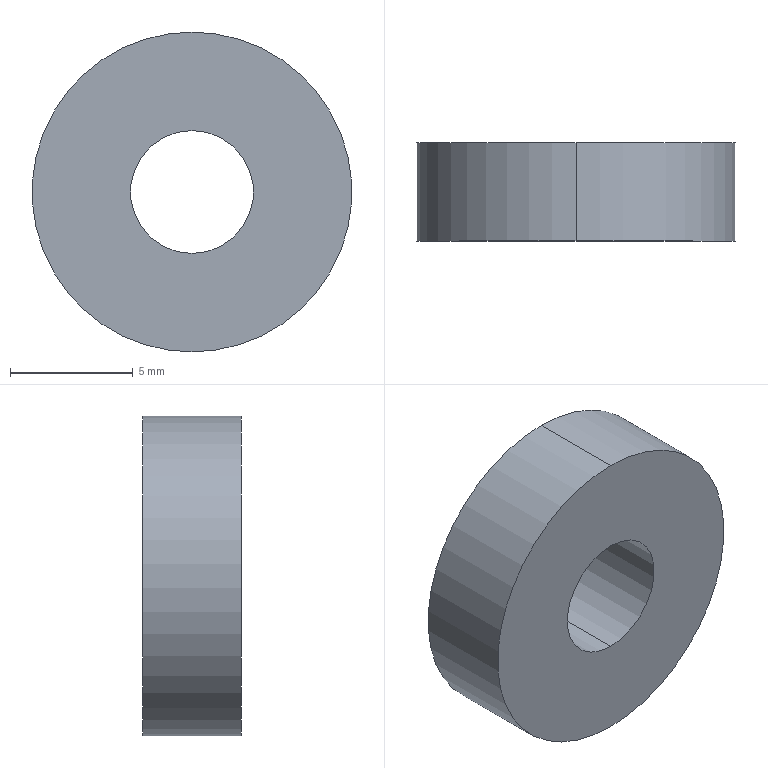Part | NX | 1 solid | 6 faces | box 13 x 4 x 13 mm | volume 452.389 mm3 | cylinder 4 | plane 2 | commonest cylinder face diameters 5 x2 13 x2
STEP:
#1=CARTESIAN_POINT('',(-123.5,286.7,-39.863));
#2=VERTEX_POINT('',#1);
#3=CARTESIAN_POINT('',(-123.5,286.7,-44.863));
#4=VERTEX_POINT('',#3);
#5=CARTESIAN_POINT('',(-123.5,286.7,-42.363));
#6=DIRECTION('',(0.,1.,0.));
#7=DIRECTION('',(0.,0.,1.));
#8=AXIS2_PLACEMENT_3D('',#5,#6,#7);
#9=CIRCLE('',#8,2.5);
#10=EDGE_CURVE('',#2,#4,#9,.T.);
#11=ORIENTED_EDGE('',*,*,#10,.F.);
#12=CARTESIAN_POINT('',(-123.5,290.7,-39.863));
#13=VERTEX_POINT('',#12);
#14=CARTESIAN_POINT('',(-123.5,290.7,-39.863));
#15=DIRECTION('',(0.,1.,0.));
#16=VECTOR('',#15,1000.);
#17=LINE('',#14,#16);
#18=EDGE_CURVE('',#2,#13,#17,.T.);
#19=ORIENTED_EDGE('',*,*,#18,.T.);
#20=CARTESIAN_POINT('',(-123.5,290.7,-44.863));
#21=VERTEX_POINT('',#20);
#22=CARTESIAN_POINT('',(-123.5,290.7,-42.363));
#23=DIRECTION('',(0.,1.,0.));
#24=DIRECTION('',(0.,0.,1.));
#25=AXIS2_PLACEMENT_3D('',#22,#23,#24);
#26=CIRCLE('',#25,2.5);
#27=EDGE_CURVE('',#13,#21,#26,.T.);
#28=ORIENTED_EDGE('',*,*,#27,.T.);
#29=CARTESIAN_POINT('',(-123.5,290.7,-44.863));
#30=DIRECTION('',(0.,1.,0.));
#31=VECTOR('',#30,1000.);
#32=LINE('',#29,#31);
#33=EDGE_CURVE('',#4,#21,#32,.T.);
#34=ORIENTED_EDGE('',*,*,#33,.F.);
#35=EDGE_LOOP('',(#11,#19,#28,#34));
#36=FACE_BOUND('',#35,.T.);
#37=CARTESIAN_POINT('',(-123.5,290.7,-42.363));
#38=DIRECTION('',(0.,1.,0.));
#39=DIRECTION('',(0.,0.,1.));
#40=AXIS2_PLACEMENT_3D('',#37,#38,#39);
#41=CYLINDRICAL_SURFACE('',#40,2.5);
#42=ADVANCED_FACE('',(#36),#41,.F.);
#43=ORIENTED_EDGE('',*,*,#18,.F.);
#44=CARTESIAN_POINT('',(-123.5,286.7,-42.363));
#45=DIRECTION('',(0.,1.,0.));
#46=DIRECTION('',(0.,0.,1.));
#47=AXIS2_PLACEMENT_3D('',#44,#45,#46);
#48=CIRCLE('',#47,2.5);
#49=EDGE_CURVE('',#4,#2,#48,.T.);
#50=ORIENTED_EDGE('',*,*,#49,.F.);
#51=ORIENTED_EDGE('',*,*,#33,.T.);
#52=CARTESIAN_POINT('',(-123.5,290.7,-42.363));
#53=DIRECTION('',(0.,1.,0.));
#54=DIRECTION('',(0.,0.,1.));
#55=AXIS2_PLACEMENT_3D('',#52,#53,#54);
#56=CIRCLE('',#55,2.5);
#57=EDGE_CURVE('',#21,#13,#56,.T.);
#58=ORIENTED_EDGE('',*,*,#57,.T.);
#59=EDGE_LOOP('',(#43,#50,#51,#58));
#60=FACE_BOUND('',#59,.T.);
#61=CARTESIAN_POINT('',(-123.5,290.7,-42.363));
#62=DIRECTION('',(0.,1.,0.));
#63=DIRECTION('',(0.,0.,1.));
#64=AXIS2_PLACEMENT_3D('',#61,#62,#63);
#65=CYLINDRICAL_SURFACE('',#64,2.5);
#66=ADVANCED_FACE('',(#60),#65,.F.);
#67=CARTESIAN_POINT('',(-123.5,286.7,-48.863));
#68=VERTEX_POINT('',#67);
#69=CARTESIAN_POINT('',(-123.5,286.7,-35.863));
#70=VERTEX_POINT('',#69);
#71=CARTESIAN_POINT('',(-123.5,286.7,-42.363));
#72=DIRECTION('',(0.,1.,0.));
#73=DIRECTION('',(0.,0.,1.));
#74=AXIS2_PLACEMENT_3D('',#71,#72,#73);
#75=CIRCLE('',#74,6.5);
#76=EDGE_CURVE('',#68,#70,#75,.T.);
#77=ORIENTED_EDGE('',*,*,#76,.T.);
#78=CARTESIAN_POINT('',(-123.5,290.7,-35.863));
#79=VERTEX_POINT('',#78);
#80=CARTESIAN_POINT('',(-123.5,290.7,-35.863));
#81=DIRECTION('',(0.,1.,0.));
#82=VECTOR('',#81,1000.);
#83=LINE('',#80,#82);
#84=EDGE_CURVE('',#70,#79,#83,.T.);
#85=ORIENTED_EDGE('',*,*,#84,.T.);
#86=CARTESIAN_POINT('',(-123.5,290.7,-48.863));
#87=VERTEX_POINT('',#86);
#88=CARTESIAN_POINT('',(-123.5,290.7,-42.363));
#89=DIRECTION('',(0.,1.,0.));
#90=DIRECTION('',(0.,0.,1.));
#91=AXIS2_PLACEMENT_3D('',#88,#89,#90);
#92=CIRCLE('',#91,6.5);
#93=EDGE_CURVE('',#87,#79,#92,.T.);
#94=ORIENTED_EDGE('',*,*,#93,.F.);
#95=CARTESIAN_POINT('',(-123.5,290.7,-48.863));
#96=DIRECTION('',(0.,1.,0.));
#97=VECTOR('',#96,1000.);
#98=LINE('',#95,#97);
#99=EDGE_CURVE('',#68,#87,#98,.T.);
#100=ORIENTED_EDGE('',*,*,#99,.F.);
#101=EDGE_LOOP('',(#77,#85,#94,#100));
#102=FACE_BOUND('',#101,.T.);
#103=CARTESIAN_POINT('',(-123.5,290.7,-42.363));
#104=DIRECTION('',(0.,1.,0.));
#105=DIRECTION('',(0.,0.,1.));
#106=AXIS2_PLACEMENT_3D('',#103,#104,#105);
#107=CYLINDRICAL_SURFACE('',#106,6.5);
#108=ADVANCED_FACE('',(#102),#107,.T.);
#109=ORIENTED_EDGE('',*,*,#84,.F.);
#110=CARTESIAN_POINT('',(-123.5,286.7,-42.363));
#111=DIRECTION('',(0.,1.,0.));
#112=DIRECTION('',(0.,0.,1.));
#113=AXIS2_PLACEMENT_3D('',#110,#111,#112);
#114=CIRCLE('',#113,6.5);
#115=EDGE_CURVE('',#70,#68,#114,.T.);
#116=ORIENTED_EDGE('',*,*,#115,.T.);
#117=ORIENTED_EDGE('',*,*,#99,.T.);
#118=CARTESIAN_POINT('',(-123.5,290.7,-42.363));
#119=DIRECTION('',(0.,1.,0.));
#120=DIRECTION('',(0.,0.,1.));
#121=AXIS2_PLACEMENT_3D('',#118,#119,#120);
#122=CIRCLE('',#121,6.5);
#123=EDGE_CURVE('',#79,#87,#122,.T.);
#124=ORIENTED_EDGE('',*,*,#123,.F.);
#125=EDGE_LOOP('',(#109,#116,#117,#124));
#126=FACE_BOUND('',#125,.T.);
#127=CARTESIAN_POINT('',(-123.5,290.7,-42.363));
#128=DIRECTION('',(0.,1.,0.));
#129=DIRECTION('',(0.,0.,1.));
#130=AXIS2_PLACEMENT_3D('',#127,#128,#129);
#131=CYLINDRICAL_SURFACE('',#130,6.5);
#132=ADVANCED_FACE('',(#126),#131,.T.);
#133=ORIENTED_EDGE('',*,*,#76,.F.);
#134=ORIENTED_EDGE('',*,*,#115,.F.);
#135=EDGE_LOOP('',(#133,#134));
#136=FACE_BOUND('',#135,.T.);
#137=ORIENTED_EDGE('',*,*,#10,.T.);
#138=ORIENTED_EDGE('',*,*,#49,.T.);
#139=EDGE_LOOP('',(#137,#138));
#140=FACE_BOUND('',#139,.T.);
#141=CARTESIAN_POINT('',(-119.723,286.7,-40.312));
#142=DIRECTION('',(0.,-1.,0.));
#143=DIRECTION('',(0.,0.,-1.));
#144=AXIS2_PLACEMENT_3D('',#141,#142,#143);
#145=PLANE('',#144);
#146=ADVANCED_FACE('',(#136,#140),#145,.T.);
#147=ORIENTED_EDGE('',*,*,#93,.T.);
#148=ORIENTED_EDGE('',*,*,#123,.T.);
#149=EDGE_LOOP('',(#147,#148));
#150=FACE_BOUND('',#149,.T.);
#151=ORIENTED_EDGE('',*,*,#27,.F.);
#152=ORIENTED_EDGE('',*,*,#57,.F.);
#153=EDGE_LOOP('',(#151,#152));
#154=FACE_BOUND('',#153,.T.);
#155=CARTESIAN_POINT('',(-119.723,290.7,-40.312));
#156=DIRECTION('',(0.,-1.,0.));
#157=DIRECTION('',(0.,0.,-1.));
#158=AXIS2_PLACEMENT_3D('',#155,#156,#157);
#159=PLANE('',#158);
#160=ADVANCED_FACE('',(#150,#154),#159,.F.);
#161=CLOSED_SHELL('',(#42,#66,#108,#132,#146,#160));
#162=MANIFOLD_SOLID_BREP('',#161);
#163=(LENGTH_UNIT()NAMED_UNIT(*)SI_UNIT(.MILLI.,.METRE.));
#164=UNCERTAINTY_MEASURE_WITH_UNIT(LENGTH_MEASURE(0.00001),#163,'','');
#165=(NAMED_UNIT(*)PLANE_ANGLE_UNIT()SI_UNIT($,.RADIAN.));
#166=(NAMED_UNIT(*)SI_UNIT($,.STERADIAN.)SOLID_ANGLE_UNIT());
#167=(GEOMETRIC_REPRESENTATION_CONTEXT(3)GLOBAL_UNCERTAINTY_ASSIGNED_CONTEXT((#164))GLOBAL_UNIT_ASSIGNED_CONTEXT((#163,#165,#166))REPRESENTATION_CONTEXT('',''));
#168=ADVANCED_BREP_SHAPE_REPRESENTATION('',(#162),#167);